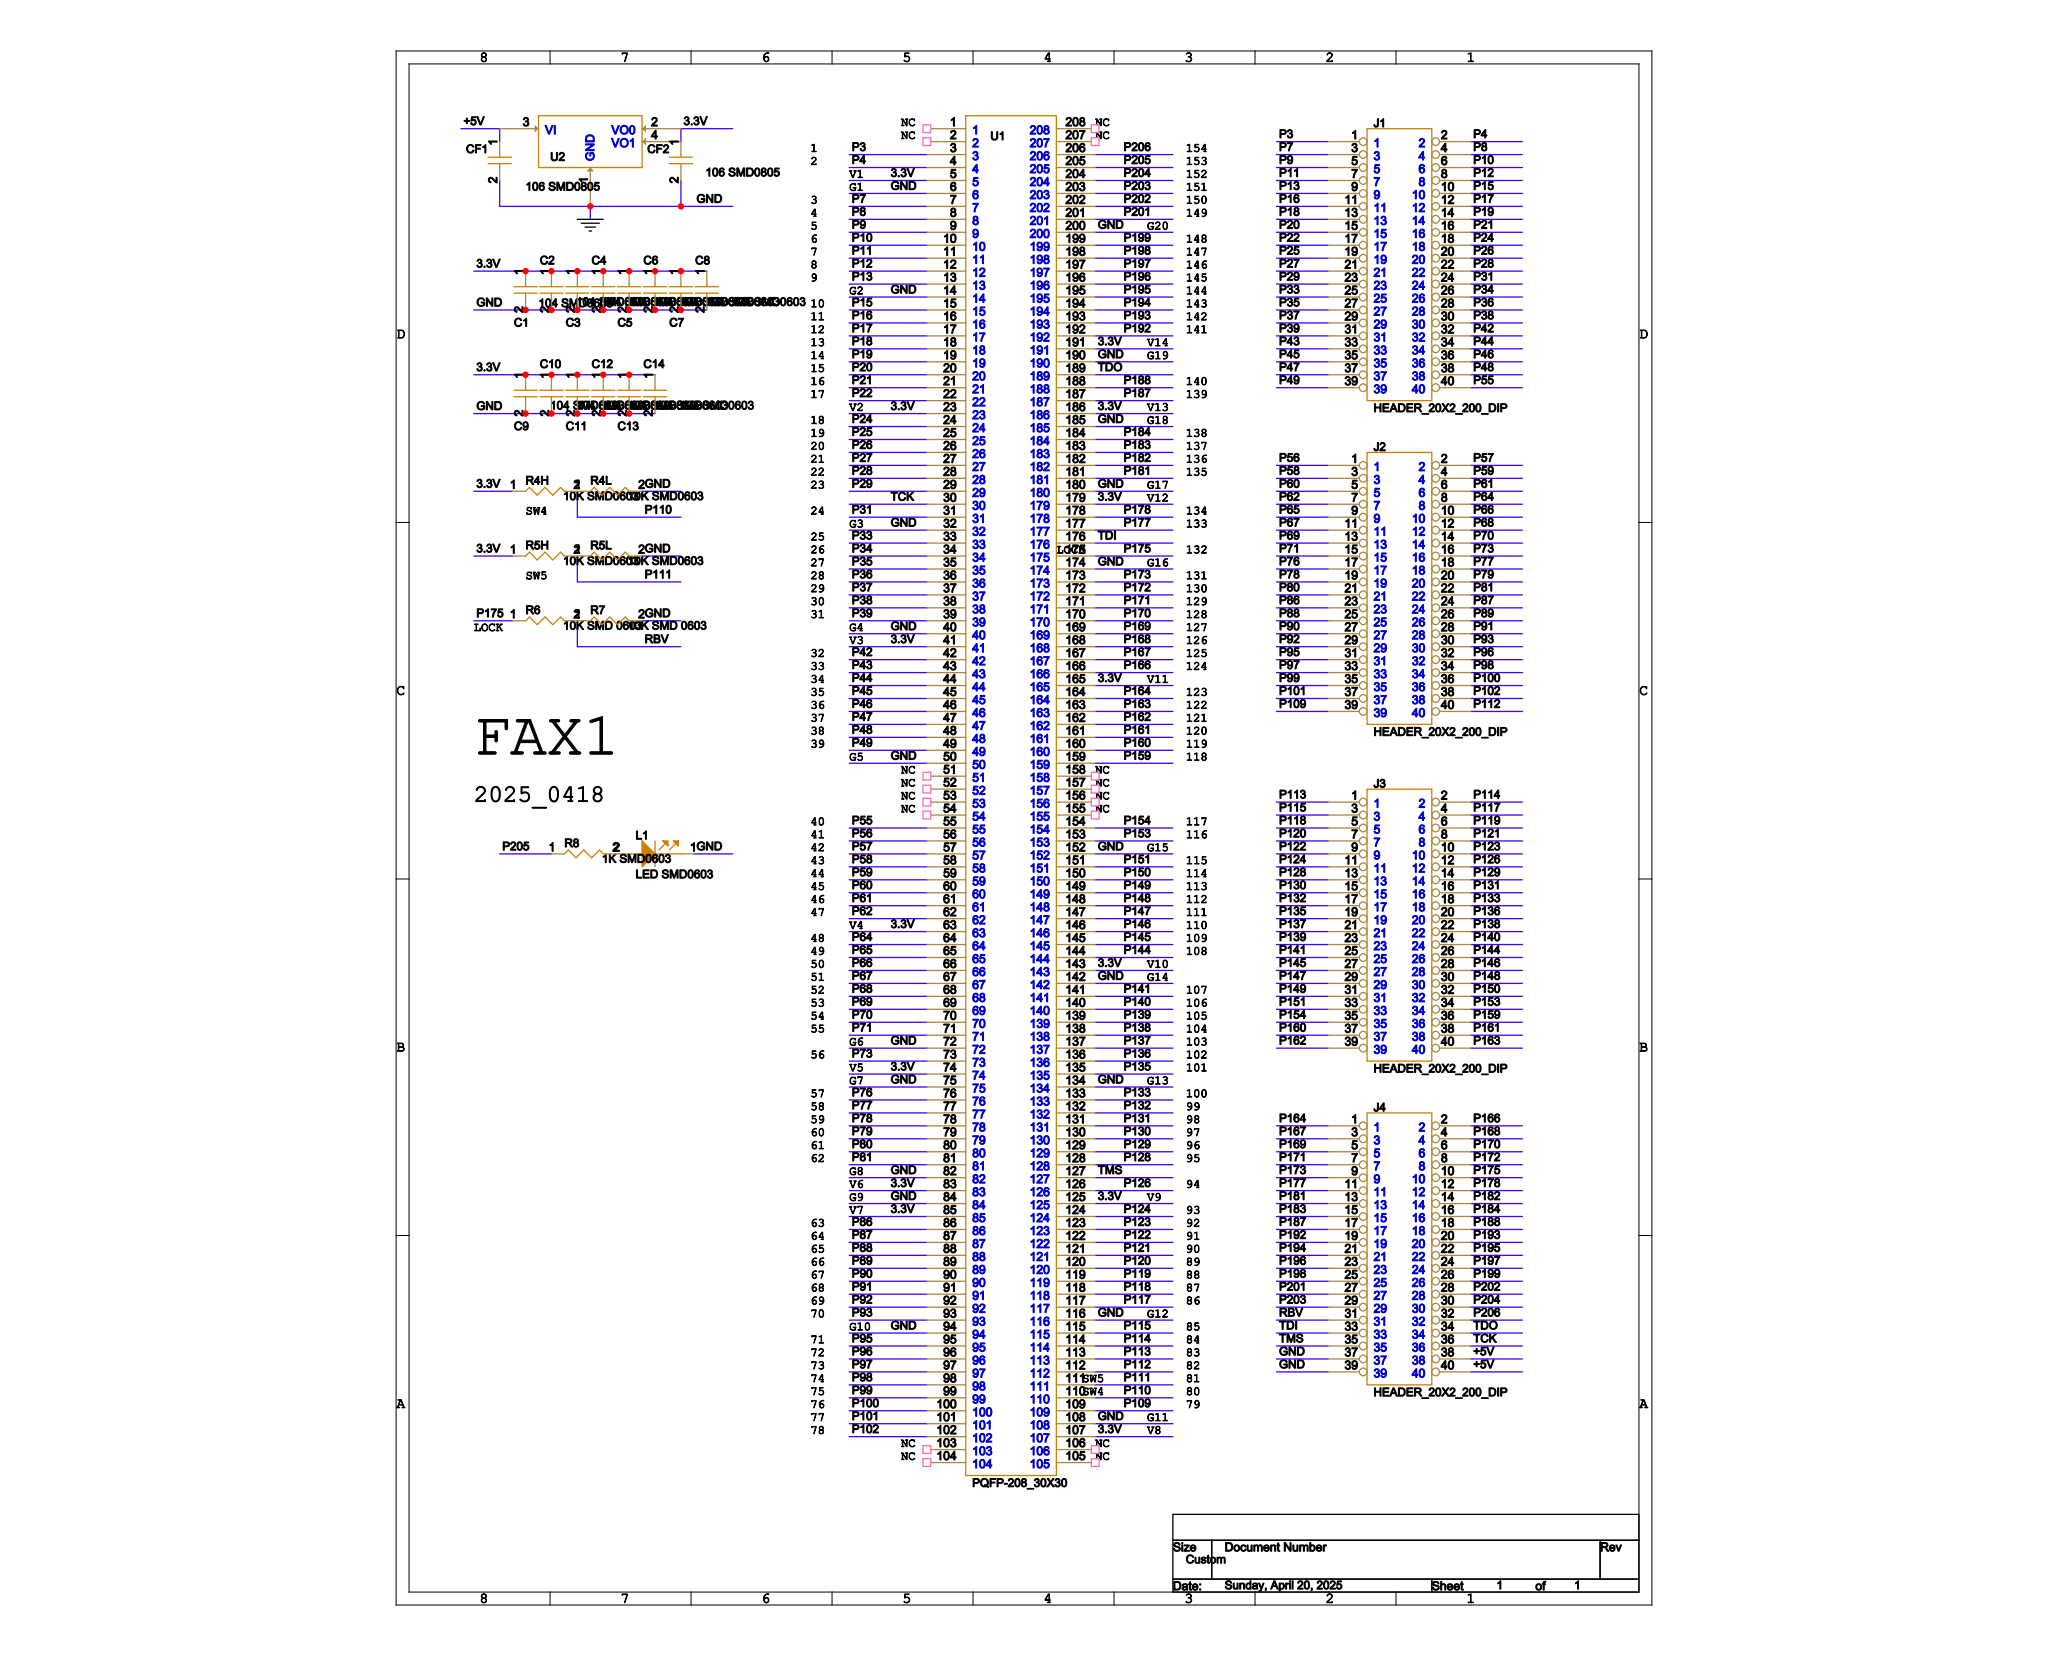Circuit board | Cadence Allegro | 30 parts | 163 nets
Bill of materials:
SYM_NAME,COMP_DEVICE_TYPE,COMP_VALUE,COMP_TOL,COMP_CLASS,REFDES
C0603,C_0_C0603_104 SMD0603,104 SMD0603,,IC,C1
C0603,C_0_C0603_104 SMD0603,104 SMD0603,,IC,C2
C0603,C_0_C0603_104 SMD0603,104 SMD0603,,IC,C3
C0603,C_0_C0603_104 SMD0603,104 SMD0603,,IC,C4
C0603,C_0_C0603_104 SMD0603,104 SMD0603,,IC,C5
C0603,C_0_C0603_104 SMD0603,104 SMD0603,,IC,C6
C0603,C_0_C0603_104 SMD0603,104 SMD0603,,IC,C7
C0603,C_0_C0603_104 SMD0603,104 SMD0603,,IC,C8
C0603,C_0_C0603_104 SMD0603,104 SMD0603,,IC,C9
C0603,C_0_C0603_104 SMD0603,104 SMD0603,,IC,C10
C0603,C_0_C0603_104 SMD0603,104 SMD0603,,IC,C11
C0603,C_0_C0603_104 SMD0603,104 SMD0603,,IC,C12
C0603,C_0_C0603_104 SMD0603,104 SMD0603,,IC,C13
C0603,C_0_C0603_104 SMD0603,104 SMD0603,,IC,C14
C0805,C_0_C0805_106 SMD0805,106 SMD0805,,IC,CF1
C0805,C_0_C0805_106 SMD0805,106 SMD0805,,IC,CF2
DIP_20X2_2MM,HEADER 20X2_1_DIP_20X2_2MM_HEAD,HEADER_20X2_200_DIP,,IC,J1
DIP_20X2_2MM,HEADER 20X2_1_DIP_20X2_2MM_HEAD,HEADER_20X2_200_DIP,,IC,J2
DIP_20X2_2MM,HEADER 20X2_1_DIP_20X2_2MM_HEAD,HEADER_20X2_200_DIP,,IC,J3
DIP_20X2_2MM,HEADER 20X2_1_DIP_20X2_2MM_HEAD,HEADER_20X2_200_DIP,,IC,J4
LED_0603,LED_1_LED_0603_LED SMD0603,LED SMD0603,,IC,L1
R0603,R_0_R0603_10K SMD0603,10K SMD0603,,IC,R4H
R0603,R_0_R0603_10K SMD0603,10K SMD0603,,IC,R4L
R0603,R_0_R0603_10K SMD0603,10K SMD0603,,IC,R5H
R0603,R_0_R0603_10K SMD0603,10K SMD0603,,IC,R5L
R0603,R_0_R0603_10K SMD 0603,10K SMD 0603,,IC,R6
R0603,R_0_R0603_10K SMD 0603,10K SMD 0603,,IC,R7
R0603,R_0_R0603_1K SMD0603,1K SMD0603,,IC,R8
PQFP-208_30X30,FPGA208_PQFP-208_30X30_PQFP-208,PQFP-208_30X30,,IC,U1
SOT-223,VOLTAGE REGULATOR_0_SOT-223_LD1,LD1117 SOT-223,,IC,U2
Netlist (net: part-pin ...):
GND: C1-2 C2-2 C3-2 C4-2 C5-2 C6-2 C7-2 C8-2 C9-2 C10-2 C11-2 C12-2 C13-2 C14-2 CF1-2 CF2-2 J4-37 J4-39 L1-1 R4L-2 R5L-2 R7-2 U1-6 U1-14 U1-32 U1-40 U1-50 U1-72 U1-75 U1-82 U1-84 U1-94 U1-108 U1-116 U1-134 U1-142 U1-152 U1-174 U1-180 U1-185 U1-190 U1-200 U2-1
N25556931801: L1-2 R8-2
+5V: CF1-1 J4-38 J4-40 U2-3
3.3V: C1-1 C2-1 C3-1 C4-1 C5-1 C6-1 C7-1 C8-1 C9-1 C10-1 C11-1 C12-1 C13-1 C14-1 CF2-1 R4H-1 R5H-1 U1-5 U1-23 U1-41 U1-63 U1-74 U1-83 U1-85 U1-107 U1-125 U1-143 U1-165 U1-179 U1-186 U1-191 U2-2 U2-4
P175: J4-10 R6-1 U1-175
RBV: J4-31 R6-2 R7-1
P10: J1-6 U1-10
P100: J2-36 U1-100
P101: J2-37 U1-101
P102: J2-38 U1-102
P109: J2-39 U1-109
P11: J1-7 U1-11
P110: R4H-2 R4L-1 U1-110
P111: R5H-2 R5L-1 U1-111
P112: J2-40 U1-112
P113: J3-1 U1-113
P114: J3-2 U1-114
P115: J3-3 U1-115
P117: J3-4 U1-117
P118: J3-5 U1-118
P119: J3-6 U1-119
P12: J1-8 U1-12
P120: J3-7 U1-120
P121: J3-8 U1-121
P122: J3-9 U1-122
P123: J3-10 U1-123
P124: J3-11 U1-124
P126: J3-12 U1-126
TMS: J4-35 U1-127
P128: J3-13 U1-128
P129: J3-14 U1-129
P13: J1-9 U1-13
P130: J3-15 U1-130
P131: J3-16 U1-131
P132: J3-17 U1-132
P133: J3-18 U1-133
P135: J3-19 U1-135
P136: J3-20 U1-136
P137: J3-21 U1-137
P138: J3-22 U1-138
P139: J3-23 U1-139
P140: J3-24 U1-140
P141: J3-25 U1-141
P144: J3-26 U1-144
P145: J3-27 U1-145
P146: J3-28 U1-146
P147: J3-29 U1-147
P148: J3-30 U1-148
P149: J3-31 U1-149
P15: J1-10 U1-15
P150: J3-32 U1-150
P151: J3-33 U1-151
P153: J3-34 U1-153
P154: J3-35 U1-154
P159: J3-36 U1-159
P16: J1-11 U1-16
P160: J3-37 U1-160
P161: J3-38 U1-161
P162: J3-39 U1-162
P163: J3-40 U1-163
P164: J4-1 U1-164
P166: J4-2 U1-166
P167: J4-3 U1-167
P168: J4-4 U1-168
P169: J4-5 U1-169
P17: J1-12 U1-17
P170: J4-6 U1-170
P171: J4-7 U1-171
P172: J4-8 U1-172
P173: J4-9 U1-173
TDI: J4-33 U1-176
P177: J4-11 U1-177
P178: J4-12 U1-178
P18: J1-13 U1-18
P181: J4-13 U1-181
P182: J4-14 U1-182
P183: J4-15 U1-183
P184: J4-16 U1-184
P187: J4-17 U1-187
P188: J4-18 U1-188
TDO: J4-34 U1-189
P19: J1-14 U1-19
P192: J4-19 U1-192
P193: J4-20 U1-193
P194: J4-21 U1-194
P195: J4-22 U1-195
P196: J4-23 U1-196
P197: J4-24 U1-197
P198: J4-25 U1-198
P199: J4-26 U1-199
P20: J1-15 U1-20
P201: J4-27 U1-201
P202: J4-28 U1-202
P203: J4-29 U1-203
P204: J4-30 U1-204
P205: R8-1 U1-205
P206: J4-32 U1-206
P21: J1-16 U1-21
P22: J1-17 U1-22
P24: J1-18 U1-24
P25: J1-19 U1-25
P26: J1-20 U1-26
P27: J1-21 U1-27
P28: J1-22 U1-28
P29: J1-23 U1-29
P3: J1-1 U1-3
TCK: J4-36 U1-30
P31: J1-24 U1-31
P33: J1-25 U1-33
P34: J1-26 U1-34
P35: J1-27 U1-35
P36: J1-28 U1-36
P37: J1-29 U1-37
P38: J1-30 U1-38
P39: J1-31 U1-39
P4: J1-2 U1-4
P42: J1-32 U1-42
P43: J1-33 U1-43
P44: J1-34 U1-44
P45: J1-35 U1-45
P46: J1-36 U1-46
P47: J1-37 U1-47
P48: J1-38 U1-48
P49: J1-39 U1-49
P55: J1-40 U1-55
P56: J2-1 U1-56
P57: J2-2 U1-57
P58: J2-3 U1-58
P59: J2-4 U1-59
P60: J2-5 U1-60
P61: J2-6 U1-61
P62: J2-7 U1-62
P64: J2-8 U1-64
P65: J2-9 U1-65
P66: J2-10 U1-66
P67: J2-11 U1-67
P68: J2-12 U1-68
P69: J2-13 U1-69
P7: J1-3 U1-7
P70: J2-14 U1-70
P71: J2-15 U1-71
P73: J2-16 U1-73
P76: J2-17 U1-76
P77: J2-18 U1-77
P78: J2-19 U1-78
P79: J2-20 U1-79
P8: J1-4 U1-8
P80: J2-21 U1-80
P81: J2-22 U1-81
P86: J2-23 U1-86
P87: J2-24 U1-87
P88: J2-25 U1-88
P89: J2-26 U1-89
P9: J1-5 U1-9
P90: J2-27 U1-90
P91: J2-28 U1-91
P92: J2-29 U1-92
P93: J2-30 U1-93
P95: J2-31 U1-95
P96: J2-32 U1-96
P97: J2-33 U1-97
P98: J2-34 U1-98
P99: J2-35 U1-99